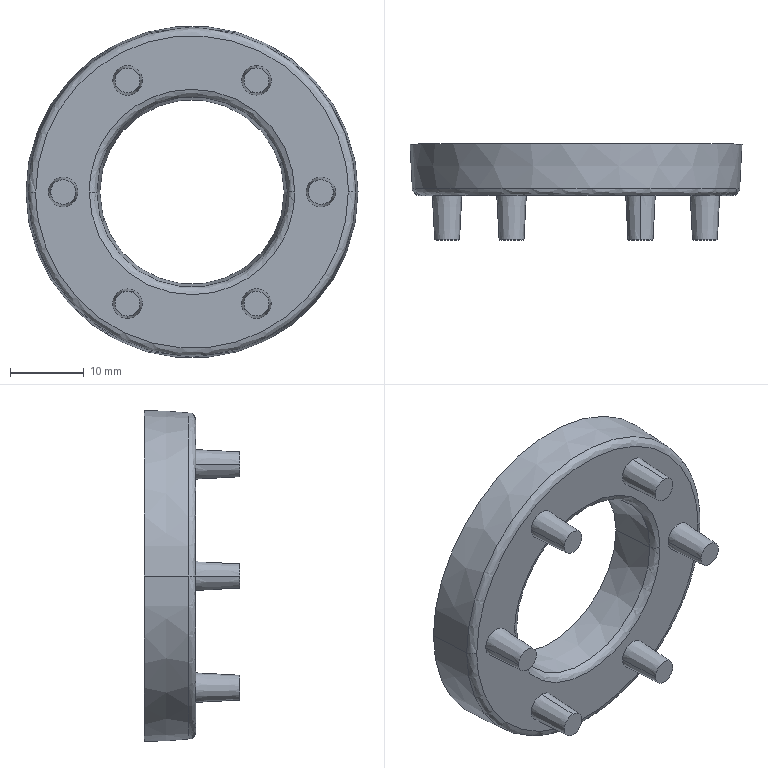Part | SolidWorks | features BaseBody 1 | 1 solid | 28 faces | box 45 x 13 x 45 mm | volume 7724 mm3 | cone 16 | plane 8 | spline 4
STEP:
#1=CARTESIAN_POINT('',(-13.922,-55.,0.));
#2=VERTEX_POINT('',#1);
#3=CARTESIAN_POINT('',(13.922,-55.,0.));
#4=VERTEX_POINT('',#3);
#5=CARTESIAN_POINT('',(-13.922,-55.,0.));
#6=CARTESIAN_POINT('',(-13.922,-55.,-27.844));
#7=CARTESIAN_POINT('',(13.922,-55.,-27.844));
#8=CARTESIAN_POINT('',(13.922,-55.,0.));
#9=(BOUNDED_CURVE()B_SPLINE_CURVE(3,(#5,#6,#7,#8),.UNSPECIFIED.,.F.,.T.)B_SPLINE_CURVE_WITH_KNOTS((4,4),(0.,0.5),.UNSPECIFIED.)CURVE()GEOMETRIC_REPRESENTATION_ITEM()RATIONAL_B_SPLINE_CURVE((1.,0.3333,0.3333,1.))REPRESENTATION_ITEM(''));
#10=EDGE_CURVE('',#2,#4,#9,.T.);
#11=ORIENTED_EDGE('',*,*,#10,.T.);
#12=CARTESIAN_POINT('',(12.924,-54.07,0.));
#13=VERTEX_POINT('',#12);
#14=CARTESIAN_POINT('',(13.922,-54.,0.));
#15=DIRECTION('',(0.,0.,-1.));
#16=DIRECTION('',(1.,0.,0.));
#17=AXIS2_PLACEMENT_3D('',#14,#15,#16);
#18=CIRCLE('',#17,1.);
#19=EDGE_CURVE('',#4,#13,#18,.T.);
#20=ORIENTED_EDGE('',*,*,#19,.T.);
#21=CARTESIAN_POINT('',(-12.924,-54.07,0.));
#22=VERTEX_POINT('',#21);
#23=CARTESIAN_POINT('',(0.,-54.07,0.));
#24=DIRECTION('',(0.,1.,0.));
#25=DIRECTION('',(1.,0.,0.));
#26=AXIS2_PLACEMENT_3D('',#23,#24,#25);
#27=CIRCLE('',#26,12.924);
#28=EDGE_CURVE('',#13,#22,#27,.T.);
#29=ORIENTED_EDGE('',*,*,#28,.T.);
#30=CARTESIAN_POINT('',(-13.922,-54.,0.));
#31=DIRECTION('',(0.,0.,1.));
#32=DIRECTION('',(-1.,0.,0.));
#33=AXIS2_PLACEMENT_3D('',#30,#31,#32);
#34=CIRCLE('',#33,1.);
#35=EDGE_CURVE('',#2,#22,#34,.T.);
#36=ORIENTED_EDGE('',*,*,#35,.F.);
#37=EDGE_LOOP('',(#11,#20,#29,#36));
#38=FACE_OUTER_BOUND('',#37,.T.);
#39=CARTESIAN_POINT('',(13.922,-55.,0.));
#40=CARTESIAN_POINT('',(13.922,-55.,-27.844));
#41=CARTESIAN_POINT('',(-13.922,-55.,-27.844));
#42=CARTESIAN_POINT('',(-13.922,-55.,0.));
#43=CARTESIAN_POINT('',(13.368,-55.,0.));
#44=CARTESIAN_POINT('',(13.368,-55.,-26.736));
#45=CARTESIAN_POINT('',(-13.368,-55.,-26.736));
#46=CARTESIAN_POINT('',(-13.368,-55.,0.));
#47=CARTESIAN_POINT('',(12.963,-54.622,0.));
#48=CARTESIAN_POINT('',(12.963,-54.622,-25.926));
#49=CARTESIAN_POINT('',(-12.963,-54.622,-25.926));
#50=CARTESIAN_POINT('',(-12.963,-54.622,0.));
#51=CARTESIAN_POINT('',(12.924,-54.07,0.));
#52=CARTESIAN_POINT('',(12.924,-54.07,-25.849));
#53=CARTESIAN_POINT('',(-12.924,-54.07,-25.849));
#54=CARTESIAN_POINT('',(-12.924,-54.07,0.));
#55=(BOUNDED_SURFACE()B_SPLINE_SURFACE(3,3,((#39,#40,#41,#42),(#43,#44,#45,#46),(#47,#48,#49,#50),(#51,#52,#53,#54)),.UNSPECIFIED.,.F.,.F.,.F.)B_SPLINE_SURFACE_WITH_KNOTS((4,4),(4,4),(0.,1.),(0.,1.),.UNSPECIFIED.)GEOMETRIC_REPRESENTATION_ITEM()RATIONAL_B_SPLINE_SURFACE(((1.,0.3333,0.3333,1.),(0.8209,0.2736,0.2736,0.8209),(0.8209,0.2736,0.2736,0.8209),(1.,0.3333,0.3333,1.)))REPRESENTATION_ITEM('')SURFACE());
#56=ADVANCED_FACE('',(#38),#55,.T.);
#57=CARTESIAN_POINT('',(22.183,-54.052,0.));
#58=VERTEX_POINT('',#57);
#59=CARTESIAN_POINT('',(-22.183,-54.052,0.));
#60=VERTEX_POINT('',#59);
#61=CARTESIAN_POINT('',(0.,-54.052,0.));
#62=DIRECTION('',(0.,1.,0.));
#63=DIRECTION('',(-1.,0.,0.));
#64=AXIS2_PLACEMENT_3D('',#61,#62,#63);
#65=CIRCLE('',#64,22.183);
#66=EDGE_CURVE('',#58,#60,#65,.T.);
#67=ORIENTED_EDGE('',*,*,#66,.F.);
#68=CARTESIAN_POINT('',(21.184,-55.,0.));
#69=VERTEX_POINT('',#68);
#70=CARTESIAN_POINT('',(21.184,-54.,0.));
#71=DIRECTION('',(0.,0.,-1.));
#72=DIRECTION('',(1.,0.,0.));
#73=AXIS2_PLACEMENT_3D('',#70,#71,#72);
#74=CIRCLE('',#73,1.);
#75=EDGE_CURVE('',#58,#69,#74,.T.);
#76=ORIENTED_EDGE('',*,*,#75,.T.);
#77=CARTESIAN_POINT('',(-21.184,-55.,0.));
#78=VERTEX_POINT('',#77);
#79=CARTESIAN_POINT('',(21.184,-55.,0.));
#80=CARTESIAN_POINT('',(21.184,-55.,-42.368));
#81=CARTESIAN_POINT('',(-21.184,-55.,-42.368));
#82=CARTESIAN_POINT('',(-21.184,-55.,0.));
#83=(BOUNDED_CURVE()B_SPLINE_CURVE(3,(#79,#80,#81,#82),.UNSPECIFIED.,.F.,.F.)B_SPLINE_CURVE_WITH_KNOTS((4,4),(0.5,1.),.UNSPECIFIED.)CURVE()GEOMETRIC_REPRESENTATION_ITEM()RATIONAL_B_SPLINE_CURVE((1.,0.3333,0.3333,1.))REPRESENTATION_ITEM(''));
#84=EDGE_CURVE('',#69,#78,#83,.T.);
#85=ORIENTED_EDGE('',*,*,#84,.T.);
#86=CARTESIAN_POINT('',(-21.184,-54.,0.));
#87=DIRECTION('',(0.,0.,1.));
#88=DIRECTION('',(-1.,0.,0.));
#89=AXIS2_PLACEMENT_3D('',#86,#87,#88);
#90=CIRCLE('',#89,1.);
#91=EDGE_CURVE('',#60,#78,#90,.T.);
#92=ORIENTED_EDGE('',*,*,#91,.F.);
#93=EDGE_LOOP('',(#67,#76,#85,#92));
#94=FACE_OUTER_BOUND('',#93,.T.);
#95=CARTESIAN_POINT('',(22.183,-54.052,0.));
#96=CARTESIAN_POINT('',(22.183,-54.052,-44.366));
#97=CARTESIAN_POINT('',(-22.183,-54.052,-44.366));
#98=CARTESIAN_POINT('',(-22.183,-54.052,0.));
#99=CARTESIAN_POINT('',(22.153,-54.613,0.));
#100=CARTESIAN_POINT('',(22.153,-54.613,-44.307));
#101=CARTESIAN_POINT('',(-22.153,-54.613,-44.307));
#102=CARTESIAN_POINT('',(-22.153,-54.613,0.));
#103=CARTESIAN_POINT('',(21.746,-55.,0.));
#104=CARTESIAN_POINT('',(21.746,-55.,-43.492));
#105=CARTESIAN_POINT('',(-21.746,-55.,-43.492));
#106=CARTESIAN_POINT('',(-21.746,-55.,0.));
#107=CARTESIAN_POINT('',(21.184,-55.,0.));
#108=CARTESIAN_POINT('',(21.184,-55.,-42.368));
#109=CARTESIAN_POINT('',(-21.184,-55.,-42.368));
#110=CARTESIAN_POINT('',(-21.184,-55.,0.));
#111=(BOUNDED_SURFACE()B_SPLINE_SURFACE(3,3,((#95,#96,#97,#98),(#99,#100,#101,#102),(#103,#104,#105,#106),(#107,#108,#109,#110)),.UNSPECIFIED.,.F.,.F.,.F.)B_SPLINE_SURFACE_WITH_KNOTS((4,4),(4,4),(0.,1.),(0.,1.),.UNSPECIFIED.)GEOMETRIC_REPRESENTATION_ITEM()RATIONAL_B_SPLINE_SURFACE(((1.,0.3333,0.3333,1.),(0.8169,0.2723,0.2723,0.8169),(0.8169,0.2723,0.2723,0.8169),(1.,0.3333,0.3333,1.)))REPRESENTATION_ITEM('')SURFACE());
#112=ADVANCED_FACE('',(#94),#111,.T.);
#113=CARTESIAN_POINT('',(-12.5,-48.,0.));
#114=VERTEX_POINT('',#113);
#115=CARTESIAN_POINT('',(12.5,-48.,0.));
#116=VERTEX_POINT('',#115);
#117=CARTESIAN_POINT('',(0.,-48.,0.));
#118=DIRECTION('',(0.,-1.,0.));
#119=DIRECTION('',(1.,0.,0.));
#120=AXIS2_PLACEMENT_3D('',#117,#118,#119);
#121=CIRCLE('',#120,12.5);
#122=EDGE_CURVE('',#114,#116,#121,.T.);
#123=ORIENTED_EDGE('',*,*,#122,.F.);
#124=CARTESIAN_POINT('',(-12.924,-54.07,0.));
#125=DIRECTION('',(-0.06976,-0.9976,0.));
#126=VECTOR('',#125,1000.);
#127=LINE('',#124,#126);
#128=EDGE_CURVE('',#114,#22,#127,.T.);
#129=ORIENTED_EDGE('',*,*,#128,.T.);
#130=ORIENTED_EDGE('',*,*,#28,.F.);
#131=CARTESIAN_POINT('',(12.924,-54.07,0.));
#132=DIRECTION('',(0.06976,-0.9976,0.));
#133=VECTOR('',#132,1000.);
#134=LINE('',#131,#133);
#135=EDGE_CURVE('',#116,#13,#134,.T.);
#136=ORIENTED_EDGE('',*,*,#135,.F.);
#137=EDGE_LOOP('',(#123,#129,#130,#136));
#138=FACE_OUTER_BOUND('',#137,.T.);
#139=CARTESIAN_POINT('',(0.,-54.07,0.));
#140=DIRECTION('',(0.,-1.,0.));
#141=DIRECTION('',(1.,0.,0.));
#142=AXIS2_PLACEMENT_3D('',#139,#140,#141);
#143=CONICAL_SURFACE('',#142,12.924,0.06981);
#144=ADVANCED_FACE('',(#138),#143,.F.);
#145=CARTESIAN_POINT('',(0.,-54.052,0.));
#146=DIRECTION('',(0.,1.,0.));
#147=DIRECTION('',(-1.,0.,0.));
#148=AXIS2_PLACEMENT_3D('',#145,#146,#147);
#149=CIRCLE('',#148,22.183);
#150=EDGE_CURVE('',#60,#58,#149,.T.);
#151=ORIENTED_EDGE('',*,*,#150,.T.);
#152=CARTESIAN_POINT('',(22.5,-48.,0.));
#153=VERTEX_POINT('',#152);
#154=CARTESIAN_POINT('',(22.5,-48.,0.));
#155=DIRECTION('',(0.05234,0.9986,0.));
#156=VECTOR('',#155,1000.);
#157=LINE('',#154,#156);
#158=EDGE_CURVE('',#58,#153,#157,.T.);
#159=ORIENTED_EDGE('',*,*,#158,.T.);
#160=CARTESIAN_POINT('',(-22.5,-48.,0.));
#161=VERTEX_POINT('',#160);
#162=CARTESIAN_POINT('',(0.,-48.,0.));
#163=DIRECTION('',(0.,1.,0.));
#164=DIRECTION('',(-1.,0.,0.));
#165=AXIS2_PLACEMENT_3D('',#162,#163,#164);
#166=CIRCLE('',#165,22.5);
#167=EDGE_CURVE('',#161,#153,#166,.T.);
#168=ORIENTED_EDGE('',*,*,#167,.F.);
#169=CARTESIAN_POINT('',(-22.5,-48.,0.));
#170=DIRECTION('',(-0.05234,0.9986,0.));
#171=VECTOR('',#170,1000.);
#172=LINE('',#169,#171);
#173=EDGE_CURVE('',#60,#161,#172,.T.);
#174=ORIENTED_EDGE('',*,*,#173,.F.);
#175=EDGE_LOOP('',(#151,#159,#168,#174));
#176=FACE_OUTER_BOUND('',#175,.T.);
#177=CARTESIAN_POINT('',(0.,-48.,0.));
#178=DIRECTION('',(0.,1.,0.));
#179=DIRECTION('',(-1.,0.,0.));
#180=AXIS2_PLACEMENT_3D('',#177,#178,#179);
#181=CONICAL_SURFACE('',#180,22.5,0.05236);
#182=ADVANCED_FACE('',(#176),#181,.T.);
#183=CARTESIAN_POINT('',(-10.422,-61.,15.133));
#184=VERTEX_POINT('',#183);
#185=CARTESIAN_POINT('',(-7.051,-61.,15.133));
#186=VERTEX_POINT('',#185);
#187=CARTESIAN_POINT('',(-8.737,-61.,15.133));
#188=DIRECTION('',(0.,1.,0.));
#189=DIRECTION('',(-1.,0.,0.));
#190=AXIS2_PLACEMENT_3D('',#187,#188,#189);
#191=CIRCLE('',#190,1.686);
#192=EDGE_CURVE('',#184,#186,#191,.T.);
#193=ORIENTED_EDGE('',*,*,#192,.T.);
#194=CARTESIAN_POINT('',(-6.737,-55.,15.133));
#195=VERTEX_POINT('',#194);
#196=CARTESIAN_POINT('',(-6.737,-55.,15.133));
#197=DIRECTION('',(0.05234,0.9986,0.));
#198=VECTOR('',#197,1000.);
#199=LINE('',#196,#198);
#200=EDGE_CURVE('',#186,#195,#199,.T.);
#201=ORIENTED_EDGE('',*,*,#200,.T.);
#202=CARTESIAN_POINT('',(-10.737,-55.,15.133));
#203=VERTEX_POINT('',#202);
#204=CARTESIAN_POINT('',(-8.737,-55.,15.133));
#205=DIRECTION('',(0.,1.,0.));
#206=DIRECTION('',(-1.,0.,0.));
#207=AXIS2_PLACEMENT_3D('',#204,#205,#206);
#208=CIRCLE('',#207,2.);
#209=EDGE_CURVE('',#203,#195,#208,.T.);
#210=ORIENTED_EDGE('',*,*,#209,.F.);
#211=CARTESIAN_POINT('',(-10.737,-55.,15.133));
#212=DIRECTION('',(-0.05234,0.9986,0.));
#213=VECTOR('',#212,1000.);
#214=LINE('',#211,#213);
#215=EDGE_CURVE('',#184,#203,#214,.T.);
#216=ORIENTED_EDGE('',*,*,#215,.F.);
#217=EDGE_LOOP('',(#193,#201,#210,#216));
#218=FACE_OUTER_BOUND('',#217,.T.);
#219=CARTESIAN_POINT('',(-8.737,-55.,15.133));
#220=DIRECTION('',(0.,1.,0.));
#221=DIRECTION('',(-1.,0.,0.));
#222=AXIS2_PLACEMENT_3D('',#219,#220,#221);
#223=CONICAL_SURFACE('',#222,2.,0.05236);
#224=ADVANCED_FACE('',(#218),#223,.T.);
#225=CARTESIAN_POINT('',(7.051,-61.,-15.133));
#226=VERTEX_POINT('',#225);
#227=CARTESIAN_POINT('',(10.422,-61.,-15.133));
#228=VERTEX_POINT('',#227);
#229=CARTESIAN_POINT('',(8.737,-61.,-15.133));
#230=DIRECTION('',(0.,1.,0.));
#231=DIRECTION('',(-1.,0.,0.));
#232=AXIS2_PLACEMENT_3D('',#229,#230,#231);
#233=CIRCLE('',#232,1.686);
#234=EDGE_CURVE('',#226,#228,#233,.T.);
#235=ORIENTED_EDGE('',*,*,#234,.T.);
#236=CARTESIAN_POINT('',(10.737,-55.,-15.133));
#237=VERTEX_POINT('',#236);
#238=CARTESIAN_POINT('',(10.737,-55.,-15.133));
#239=DIRECTION('',(0.05234,0.9986,0.));
#240=VECTOR('',#239,1000.);
#241=LINE('',#238,#240);
#242=EDGE_CURVE('',#228,#237,#241,.T.);
#243=ORIENTED_EDGE('',*,*,#242,.T.);
#244=CARTESIAN_POINT('',(6.737,-55.,-15.133));
#245=VERTEX_POINT('',#244);
#246=CARTESIAN_POINT('',(8.737,-55.,-15.133));
#247=DIRECTION('',(0.,1.,0.));
#248=DIRECTION('',(-1.,0.,0.));
#249=AXIS2_PLACEMENT_3D('',#246,#247,#248);
#250=CIRCLE('',#249,2.);
#251=EDGE_CURVE('',#245,#237,#250,.T.);
#252=ORIENTED_EDGE('',*,*,#251,.F.);
#253=CARTESIAN_POINT('',(6.737,-55.,-15.133));
#254=DIRECTION('',(-0.05234,0.9986,0.));
#255=VECTOR('',#254,1000.);
#256=LINE('',#253,#255);
#257=EDGE_CURVE('',#226,#245,#256,.T.);
#258=ORIENTED_EDGE('',*,*,#257,.F.);
#259=EDGE_LOOP('',(#235,#243,#252,#258));
#260=FACE_OUTER_BOUND('',#259,.T.);
#261=CARTESIAN_POINT('',(8.737,-55.,-15.133));
#262=DIRECTION('',(0.,1.,0.));
#263=DIRECTION('',(-1.,0.,0.));
#264=AXIS2_PLACEMENT_3D('',#261,#262,#263);
#265=CONICAL_SURFACE('',#264,2.,0.05236);
#266=ADVANCED_FACE('',(#260),#265,.T.);
#267=CARTESIAN_POINT('',(8.737,-61.,16.818));
#268=VERTEX_POINT('',#267);
#269=CARTESIAN_POINT('',(8.737,-61.,13.447));
#270=VERTEX_POINT('',#269);
#271=CARTESIAN_POINT('',(8.737,-61.,15.133));
#272=DIRECTION('',(0.,1.,0.));
#273=DIRECTION('',(0.,0.,1.));
#274=AXIS2_PLACEMENT_3D('',#271,#272,#273);
#275=CIRCLE('',#274,1.686);
#276=EDGE_CURVE('',#268,#270,#275,.T.);
#277=ORIENTED_EDGE('',*,*,#276,.T.);
#278=CARTESIAN_POINT('',(8.737,-55.,13.133));
#279=VERTEX_POINT('',#278);
#280=CARTESIAN_POINT('',(8.737,-55.,13.133));
#281=DIRECTION('',(0.,0.9986,-0.05234));
#282=VECTOR('',#281,1000.);
#283=LINE('',#280,#282);
#284=EDGE_CURVE('',#270,#279,#283,.T.);
#285=ORIENTED_EDGE('',*,*,#284,.T.);
#286=CARTESIAN_POINT('',(8.737,-55.,17.133));
#287=VERTEX_POINT('',#286);
#288=CARTESIAN_POINT('',(8.737,-55.,15.133));
#289=DIRECTION('',(0.,1.,0.));
#290=DIRECTION('',(0.,0.,1.));
#291=AXIS2_PLACEMENT_3D('',#288,#289,#290);
#292=CIRCLE('',#291,2.);
#293=EDGE_CURVE('',#287,#279,#292,.T.);
#294=ORIENTED_EDGE('',*,*,#293,.F.);
#295=CARTESIAN_POINT('',(8.737,-55.,17.133));
#296=DIRECTION('',(0.,0.9986,0.05234));
#297=VECTOR('',#296,1000.);
#298=LINE('',#295,#297);
#299=EDGE_CURVE('',#268,#287,#298,.T.);
#300=ORIENTED_EDGE('',*,*,#299,.F.);
#301=EDGE_LOOP('',(#277,#285,#294,#300));
#302=FACE_OUTER_BOUND('',#301,.T.);
#303=CARTESIAN_POINT('',(8.737,-55.,15.133));
#304=DIRECTION('',(0.,1.,0.));
#305=DIRECTION('',(0.,0.,1.));
#306=AXIS2_PLACEMENT_3D('',#303,#304,#305);
#307=CONICAL_SURFACE('',#306,2.,0.05236);
#308=ADVANCED_FACE('',(#302),#307,.T.);
#309=CARTESIAN_POINT('',(15.788,-61.,0.));
#310=VERTEX_POINT('',#309);
#311=CARTESIAN_POINT('',(19.159,-61.,0.));
#312=VERTEX_POINT('',#311);
#313=CARTESIAN_POINT('',(17.474,-61.,0.));
#314=DIRECTION('',(0.,1.,0.));
#315=DIRECTION('',(-1.,0.,0.));
#316=AXIS2_PLACEMENT_3D('',#313,#314,#315);
#317=CIRCLE('',#316,1.686);
#318=EDGE_CURVE('',#310,#312,#317,.T.);
#319=ORIENTED_EDGE('',*,*,#318,.T.);
#320=CARTESIAN_POINT('',(19.474,-55.,0.));
#321=VERTEX_POINT('',#320);
#322=CARTESIAN_POINT('',(19.474,-55.,0.));
#323=DIRECTION('',(0.05234,0.9986,0.));
#324=VECTOR('',#323,1000.);
#325=LINE('',#322,#324);
#326=EDGE_CURVE('',#312,#321,#325,.T.);
#327=ORIENTED_EDGE('',*,*,#326,.T.);
#328=CARTESIAN_POINT('',(15.474,-55.,0.));
#329=VERTEX_POINT('',#328);
#330=CARTESIAN_POINT('',(17.474,-55.,0.));
#331=DIRECTION('',(0.,1.,0.));
#332=DIRECTION('',(-1.,0.,0.));
#333=AXIS2_PLACEMENT_3D('',#330,#331,#332);
#334=CIRCLE('',#333,2.);
#335=EDGE_CURVE('',#329,#321,#334,.T.);
#336=ORIENTED_EDGE('',*,*,#335,.F.);
#337=CARTESIAN_POINT('',(15.474,-55.,0.));
#338=DIRECTION('',(-0.05234,0.9986,0.));
#339=VECTOR('',#338,1000.);
#340=LINE('',#337,#339);
#341=EDGE_CURVE('',#310,#329,#340,.T.);
#342=ORIENTED_EDGE('',*,*,#341,.F.);
#343=EDGE_LOOP('',(#319,#327,#336,#342));
#344=FACE_OUTER_BOUND('',#343,.T.);
#345=CARTESIAN_POINT('',(17.474,-55.,0.));
#346=DIRECTION('',(0.,1.,0.));
#347=DIRECTION('',(-1.,0.,0.));
#348=AXIS2_PLACEMENT_3D('',#345,#346,#347);
#349=CONICAL_SURFACE('',#348,2.,0.05236);
#350=ADVANCED_FACE('',(#344),#349,.T.);
#351=CARTESIAN_POINT('',(-19.159,-61.,0.));
#352=VERTEX_POINT('',#351);
#353=CARTESIAN_POINT('',(-15.788,-61.,0.));
#354=VERTEX_POINT('',#353);
#355=CARTESIAN_POINT('',(-17.474,-61.,0.));
#356=DIRECTION('',(0.,1.,0.));
#357=DIRECTION('',(-1.,0.,0.));
#358=AXIS2_PLACEMENT_3D('',#355,#356,#357);
#359=CIRCLE('',#358,1.686);
#360=EDGE_CURVE('',#352,#354,#359,.T.);
#361=ORIENTED_EDGE('',*,*,#360,.T.);
#362=CARTESIAN_POINT('',(-15.474,-55.,0.));
#363=VERTEX_POINT('',#362);
#364=CARTESIAN_POINT('',(-15.474,-55.,0.));
#365=DIRECTION('',(0.05234,0.9986,0.));
#366=VECTOR('',#365,1000.);
#367=LINE('',#364,#366);
#368=EDGE_CURVE('',#354,#363,#367,.T.);
#369=ORIENTED_EDGE('',*,*,#368,.T.);
#370=CARTESIAN_POINT('',(-19.474,-55.,0.));
#371=VERTEX_POINT('',#370);
#372=CARTESIAN_POINT('',(-17.474,-55.,0.));
#373=DIRECTION('',(0.,1.,0.));
#374=DIRECTION('',(-1.,0.,0.));
#375=AXIS2_PLACEMENT_3D('',#372,#373,#374);
#376=CIRCLE('',#375,2.);
#377=EDGE_CURVE('',#371,#363,#376,.T.);
#378=ORIENTED_EDGE('',*,*,#377,.F.);
#379=CARTESIAN_POINT('',(-19.474,-55.,0.));
#380=DIRECTION('',(-0.05234,0.9986,0.));
#381=VECTOR('',#380,1000.);
#382=LINE('',#379,#381);
#383=EDGE_CURVE('',#352,#371,#382,.T.);
#384=ORIENTED_EDGE('',*,*,#383,.F.);
#385=EDGE_LOOP('',(#361,#369,#378,#384));
#386=FACE_OUTER_BOUND('',#385,.T.);
#387=CARTESIAN_POINT('',(-17.474,-55.,0.));
#388=DIRECTION('',(0.,1.,0.));
#389=DIRECTION('',(-1.,0.,0.));
#390=AXIS2_PLACEMENT_3D('',#387,#388,#389);
#391=CONICAL_SURFACE('',#390,2.,0.05236);
#392=ADVANCED_FACE('',(#386),#391,.T.);
#393=CARTESIAN_POINT('',(-8.737,-61.,-13.447));
#394=VERTEX_POINT('',#393);
#395=CARTESIAN_POINT('',(-8.737,-61.,-16.818));
#396=VERTEX_POINT('',#395);
#397=CARTESIAN_POINT('',(-8.737,-61.,-15.133));
#398=DIRECTION('',(0.,1.,0.));
#399=DIRECTION('',(0.,0.,1.));
#400=AXIS2_PLACEMENT_3D('',#397,#398,#399);
#401=CIRCLE('',#400,1.686);
#402=EDGE_CURVE('',#394,#396,#401,.T.);
#403=ORIENTED_EDGE('',*,*,#402,.T.);
#404=CARTESIAN_POINT('',(-8.737,-55.,-17.133));
#405=VERTEX_POINT('',#404);
#406=CARTESIAN_POINT('',(-8.737,-55.,-17.133));
#407=DIRECTION('',(0.,0.9986,-0.05234));
#408=VECTOR('',#407,1000.);
#409=LINE('',#406,#408);
#410=EDGE_CURVE('',#396,#405,#409,.T.);
#411=ORIENTED_EDGE('',*,*,#410,.T.);
#412=CARTESIAN_POINT('',(-8.737,-55.,-13.133));
#413=VERTEX_POINT('',#412);
#414=CARTESIAN_POINT('',(-8.737,-55.,-15.133));
#415=DIRECTION('',(0.,1.,0.));
#416=DIRECTION('',(0.,0.,1.));
#417=AXIS2_PLACEMENT_3D('',#414,#415,#416);
#418=CIRCLE('',#417,2.);
#419=EDGE_CURVE('',#413,#405,#418,.T.);
#420=ORIENTED_EDGE('',*,*,#419,.F.);
#421=CARTESIAN_POINT('',(-8.737,-55.,-13.133));
#422=DIRECTION('',(0.,0.9986,0.05234));
#423=VECTOR('',#422,1000.);
#424=LINE('',#421,#423);
#425=EDGE_CURVE('',#394,#413,#424,.T.);
#426=ORIENTED_EDGE('',*,*,#425,.F.);
#427=EDGE_LOOP('',(#403,#411,#420,#426));
#428=FACE_OUTER_BOUND('',#427,.T.);
#429=CARTESIAN_POINT('',(-8.737,-55.,-15.133));
#430=DIRECTION('',(0.,1.,0.));
#431=DIRECTION('',(0.,0.,1.));
#432=AXIS2_PLACEMENT_3D('',#429,#430,#431);
#433=CONICAL_SURFACE('',#432,2.,0.05236);
#434=ADVANCED_FACE('',(#428),#433,.T.);
#435=CARTESIAN_POINT('',(0.,-48.,0.));
#436=DIRECTION('',(0.,-1.,0.));
#437=DIRECTION('',(1.,0.,0.));
#438=AXIS2_PLACEMENT_3D('',#435,#436,#437);
#439=CIRCLE('',#438,12.5);
#440=EDGE_CURVE('',#116,#114,#439,.T.);
#441=ORIENTED_EDGE('',*,*,#440,.T.);
#442=ORIENTED_EDGE('',*,*,#122,.T.);
#443=EDGE_LOOP('',(#441,#442));
#444=FACE_BOUND('',#443,.T.);
#445=ORIENTED_EDGE('',*,*,#167,.T.);
#446=CARTESIAN_POINT('',(0.,-48.,0.));
#447=DIRECTION('',(0.,1.,0.));
#448=DIRECTION('',(-1.,0.,0.));
#449=AXIS2_PLACEMENT_3D('',#446,#447,#448);
#450=CIRCLE('',#449,22.5);
#451=EDGE_CURVE('',#153,#161,#450,.T.);
#452=ORIENTED_EDGE('',*,*,#451,.T.);
#453=EDGE_LOOP('',(#445,#452));
#454=FACE_OUTER_BOUND('',#453,.T.);
#455=CARTESIAN_POINT('',(0.,-48.,-12.5));
#456=DIRECTION('',(0.,1.,0.));
#457=DIRECTION('',(0.,0.,1.));
#458=AXIS2_PLACEMENT_3D('',#455,#456,#457);
#459=PLANE('',#458);
#460=ADVANCED_FACE('',(#444,#454),#459,.T.);
#461=ORIENTED_EDGE('',*,*,#128,.F.);
#462=ORIENTED_EDGE('',*,*,#440,.F.);
#463=ORIENTED_EDGE('',*,*,#135,.T.);
#464=CARTESIAN_POINT('',(0.,-54.07,0.));
#465=DIRECTION('',(0.,1.,0.));
#466=DIRECTION('',(1.,0.,0.));
#467=AXIS2_PLACEMENT_3D('',#464,#465,#466);
#468=CIRCLE('',#467,12.924);
#469=EDGE_CURVE('',#22,#13,#468,.T.);
#470=ORIENTED_EDGE('',*,*,#469,.F.);
#471=EDGE_LOOP('',(#461,#462,#463,#470));
#472=FACE_OUTER_BOUND('',#471,.T.);
#473=CARTESIAN_POINT('',(0.,-54.07,0.));
#474=DIRECTION('',(0.,-1.,0.));
#475=DIRECTION('',(1.,0.,0.));
#476=AXIS2_PLACEMENT_3D('',#473,#474,#475);
#477=CONICAL_SURFACE('',#476,12.924,0.06981);
#478=ADVANCED_FACE('',(#472),#477,.F.);
#479=ORIENTED_EDGE('',*,*,#158,.F.);
#480=ORIENTED_EDGE('',*,*,#66,.T.);
#481=ORIENTED_EDGE('',*,*,#173,.T.);
#482=ORIENTED_EDGE('',*,*,#451,.F.);
#483=EDGE_LOOP('',(#479,#480,#481,#482));
#484=FACE_OUTER_BOUND('',#483,.T.);
#485=CARTESIAN_POINT('',(0.,-48.,0.));
#486=DIRECTION('',(0.,1.,0.));
#487=DIRECTION('',(-1.,0.,0.));
#488=AXIS2_PLACEMENT_3D('',#485,#486,#487);
#489=CONICAL_SURFACE('',#488,22.5,0.05236);
#490=ADVANCED_FACE('',(#484),#489,.T.);
#491=ORIENTED_EDGE('',*,*,#19,.F.);
#492=CARTESIAN_POINT('',(13.922,-55.,0.));
#493=CARTESIAN_POINT('',(13.922,-55.,27.844));
#494=CARTESIAN_POINT('',(-13.922,-55.,27.844));
#495=CARTESIAN_POINT('',(-13.922,-55.,0.));
#496=(BOUNDED_CURVE()B_SPLINE_CURVE(3,(#492,#493,#494,#495),.UNSPECIFIED.,.F.,.F.)B_SPLINE_CURVE_WITH_KNOTS((4,4),(0.5,1.),.UNSPECIFIED.)CURVE()GEOMETRIC_REPRESENTATION_ITEM()RATIONAL_B_SPLINE_CURVE((1.,0.3333,0.3333,1.))REPRESENTATION_ITEM(''));
#497=EDGE_CURVE('',#4,#2,#496,.T.);
#498=ORIENTED_EDGE('',*,*,#497,.T.);
#499=ORIENTED_EDGE('',*,*,#35,.T.);
#500=ORIENTED_EDGE('',*,*,#469,.T.);
#501=EDGE_LOOP('',(#491,#498,#499,#500));
#502=FACE_OUTER_BOUND('',#501,.T.);
#503=CARTESIAN_POINT('',(-13.922,-55.,0.));
#504=CARTESIAN_POINT('',(-13.922,-55.,27.844));
#505=CARTESIAN_POINT('',(13.922,-55.,27.844));
#506=CARTESIAN_POINT('',(13.922,-55.,0.));
#507=CARTESIAN_POINT('',(-13.368,-55.,0.));
#508=CARTESIAN_POINT('',(-13.368,-55.,26.736));
#509=CARTESIAN_POINT('',(13.368,-55.,26.736));
#510=CARTESIAN_POINT('',(13.368,-55.,0.));
#511=CARTESIAN_POINT('',(-12.963,-54.622,0.));
#512=CARTESIAN_POINT('',(-12.963,-54.622,25.926));
#513=CARTESIAN_POINT('',(12.963,-54.622,25.926));
#514=CARTESIAN_POINT('',(12.963,-54.622,0.));
#515=CARTESIAN_POINT('',(-12.924,-54.07,0.));
#516=CARTESIAN_POINT('',(-12.924,-54.07,25.849));
#517=CARTESIAN_POINT('',(12.924,-54.07,25.849));
#518=CARTESIAN_POINT('',(12.924,-54.07,0.));
#519=(BOUNDED_SURFACE()B_SPLINE_SURFACE(3,3,((#503,#504,#505,#506),(#507,#508,#509,#510),(#511,#512,#513,#514),(#515,#516,#517,#518)),.UNSPECIFIED.,.F.,.F.,.F.)B_SPLINE_SURFACE_WITH_KNOTS((4,4),(4,4),(0.,1.),(0.,1.),.UNSPECIFIED.)GEOMETRIC_REPRESENTATION_ITEM()RATIONAL_B_SPLINE_SURFACE(((1.,0.3333,0.3333,1.),(0.8209,0.2736,0.2736,0.8209),(0.8209,0.2736,0.2736,0.8209),(1.,0.3333,0.3333,1.)))REPRESENTATION_ITEM('')SURFACE());
#520=ADVANCED_FACE('',(#502),#519,.T.);
#521=ORIENTED_EDGE('',*,*,#75,.F.);
#522=ORIENTED_EDGE('',*,*,#150,.F.);
#523=ORIENTED_EDGE('',*,*,#91,.T.);
#524=CARTESIAN_POINT('',(-21.184,-55.,0.));
#525=CARTESIAN_POINT('',(-21.184,-55.,42.368));
#526=CARTESIAN_POINT('',(21.184,-55.,42.368));
#527=CARTESIAN_POINT('',(21.184,-55.,0.));
#528=(BOUNDED_CURVE()B_SPLINE_CURVE(3,(#524,#525,#526,#527),.UNSPECIFIED.,.F.,.F.)B_SPLINE_CURVE_WITH_KNOTS((4,4),(0.,0.5),.UNSPECIFIED.)CURVE()GEOMETRIC_REPRESENTATION_ITEM()RATIONAL_B_SPLINE_CURVE((1.,0.3333,0.3333,1.))REPRESENTATION_ITEM(''));
#529=EDGE_CURVE('',#78,#69,#528,.T.);
#530=ORIENTED_EDGE('',*,*,#529,.T.);
#531=EDGE_LOOP('',(#521,#522,#523,#530));
#532=FACE_OUTER_BOUND('',#531,.T.);
#533=CARTESIAN_POINT('',(-22.183,-54.052,0.));
#534=CARTESIAN_POINT('',(-22.183,-54.052,44.366));
#535=CARTESIAN_POINT('',(22.183,-54.052,44.366));
#536=CARTESIAN_POINT('',(22.183,-54.052,0.));
#537=CARTESIAN_POINT('',(-22.153,-54.613,0.));
#538=CARTESIAN_POINT('',(-22.153,-54.613,44.307));
#539=CARTESIAN_POINT('',(22.153,-54.613,44.307));
#540=CARTESIAN_POINT('',(22.153,-54.613,0.));
#541=CARTESIAN_POINT('',(-21.746,-55.,0.));
#542=CARTESIAN_POINT('',(-21.746,-55.,43.492));
#543=CARTESIAN_POINT('',(21.746,-55.,43.492));
#544=CARTESIAN_POINT('',(21.746,-55.,0.));
#545=CARTESIAN_POINT('',(-21.184,-55.,0.));
#546=CARTESIAN_POINT('',(-21.184,-55.,42.368));
#547=CARTESIAN_POINT('',(21.184,-55.,42.368));
#548=CARTESIAN_POINT('',(21.184,-55.,0.));
#549=(BOUNDED_SURFACE()B_SPLINE_SURFACE(3,3,((#533,#534,#535,#536),(#537,#538,#539,#540),(#541,#542,#543,#544),(#545,#546,#547,#548)),.UNSPECIFIED.,.F.,.F.,.F.)B_SPLINE_SURFACE_WITH_KNOTS((4,4),(4,4),(0.,1.),(0.,1.),.UNSPECIFIED.)GEOMETRIC_REPRESENTATION_ITEM()RATIONAL_B_SPLINE_SURFACE(((1.,0.3333,0.3333,1.),(0.8169,0.2723,0.2723,0.8169),(0.8169,0.2723,0.2723,0.8169),(1.,0.3333,0.3333,1.)))REPRESENTATION_ITEM('')SURFACE());
#550=ADVANCED_FACE('',(#532),#549,.T.);
#551=ORIENTED_EDGE('',*,*,#529,.F.);
#552=ORIENTED_EDGE('',*,*,#84,.F.);
#553=EDGE_LOOP('',(#551,#552));
#554=FACE_OUTER_BOUND('',#553,.T.);
#555=ORIENTED_EDGE('',*,*,#10,.F.);
#556=ORIENTED_EDGE('',*,*,#497,.F.);
#557=EDGE_LOOP('',(#555,#556));
#558=FACE_BOUND('',#557,.T.);
#559=ORIENTED_EDGE('',*,*,#209,.T.);
#560=CARTESIAN_POINT('',(-8.737,-55.,15.133));
#561=DIRECTION('',(0.,1.,0.));
#562=DIRECTION('',(-1.,0.,0.));
#563=AXIS2_PLACEMENT_3D('',#560,#561,#562);
#564=CIRCLE('',#563,2.);
#565=EDGE_CURVE('',#195,#203,#564,.T.);
#566=ORIENTED_EDGE('',*,*,#565,.T.);
#567=EDGE_LOOP('',(#559,#566));
#568=FACE_BOUND('',#567,.T.);
#569=ORIENTED_EDGE('',*,*,#251,.T.);
#570=CARTESIAN_POINT('',(8.737,-55.,-15.133));
#571=DIRECTION('',(0.,1.,0.));
#572=DIRECTION('',(-1.,0.,0.));
#573=AXIS2_PLACEMENT_3D('',#570,#571,#572);
#574=CIRCLE('',#573,2.);
#575=EDGE_CURVE('',#237,#245,#574,.T.);
#576=ORIENTED_EDGE('',*,*,#575,.T.);
#577=EDGE_LOOP('',(#569,#576));
#578=FACE_BOUND('',#577,.T.);
#579=ORIENTED_EDGE('',*,*,#293,.T.);
#580=CARTESIAN_POINT('',(8.737,-55.,15.133));
#581=DIRECTION('',(0.,1.,0.));
#582=DIRECTION('',(0.,0.,1.));
#583=AXIS2_PLACEMENT_3D('',#580,#581,#582);
#584=CIRCLE('',#583,2.);
#585=EDGE_CURVE('',#279,#287,#584,.T.);
#586=ORIENTED_EDGE('',*,*,#585,.T.);
#587=EDGE_LOOP('',(#579,#586));
#588=FACE_BOUND('',#587,.T.);
#589=ORIENTED_EDGE('',*,*,#335,.T.);
#590=CARTESIAN_POINT('',(17.474,-55.,0.));
#591=DIRECTION('',(0.,1.,0.));
#592=DIRECTION('',(-1.,0.,0.));
#593=AXIS2_PLACEMENT_3D('',#590,#591,#592);
#594=CIRCLE('',#593,2.);
#595=EDGE_CURVE('',#321,#329,#594,.T.);
#596=ORIENTED_EDGE('',*,*,#595,.T.);
#597=EDGE_LOOP('',(#589,#596));
#598=FACE_BOUND('',#597,.T.);
#599=ORIENTED_EDGE('',*,*,#377,.T.);
#600=CARTESIAN_POINT('',(-17.474,-55.,0.));
#601=DIRECTION('',(0.,1.,0.));
#602=DIRECTION('',(-1.,0.,0.));
#603=AXIS2_PLACEMENT_3D('',#600,#601,#602);
#604=CIRCLE('',#603,2.);
#605=EDGE_CURVE('',#363,#371,#604,.T.);
#606=ORIENTED_EDGE('',*,*,#605,.T.);
#607=EDGE_LOOP('',(#599,#606));
#608=FACE_BOUND('',#607,.T.);
#609=ORIENTED_EDGE('',*,*,#419,.T.);
#610=CARTESIAN_POINT('',(-8.737,-55.,-15.133));
#611=DIRECTION('',(0.,1.,0.));
#612=DIRECTION('',(0.,0.,1.));
#613=AXIS2_PLACEMENT_3D('',#610,#611,#612);
#614=CIRCLE('',#613,2.);
#615=EDGE_CURVE('',#405,#413,#614,.T.);
#616=ORIENTED_EDGE('',*,*,#615,.T.);
#617=EDGE_LOOP('',(#609,#616));
#618=FACE_BOUND('',#617,.T.);
#619=CARTESIAN_POINT('',(0.,-55.,-21.184));
#620=DIRECTION('',(0.,-1.,0.));
#621=DIRECTION('',(0.,0.,-1.));
#622=AXIS2_PLACEMENT_3D('',#619,#620,#621);
#623=PLANE('',#622);
#624=ADVANCED_FACE('',(#554,#558,#568,#578,#588,#598,#608,#618),#623,.T.);
#625=ORIENTED_EDGE('',*,*,#200,.F.);
#626=CARTESIAN_POINT('',(-8.737,-61.,15.133));
#627=DIRECTION('',(0.,1.,0.));
#628=DIRECTION('',(-1.,0.,0.));
#629=AXIS2_PLACEMENT_3D('',#626,#627,#628);
#630=CIRCLE('',#629,1.686);
#631=EDGE_CURVE('',#186,#184,#630,.T.);
#632=ORIENTED_EDGE('',*,*,#631,.T.);
#633=ORIENTED_EDGE('',*,*,#215,.T.);
#634=ORIENTED_EDGE('',*,*,#565,.F.);
#635=EDGE_LOOP('',(#625,#632,#633,#634));
#636=FACE_OUTER_BOUND('',#635,.T.);
#637=CARTESIAN_POINT('',(-8.737,-55.,15.133));
#638=DIRECTION('',(0.,1.,0.));
#639=DIRECTION('',(-1.,0.,0.));
#640=AXIS2_PLACEMENT_3D('',#637,#638,#639);
#641=CONICAL_SURFACE('',#640,2.,0.05236);
#642=ADVANCED_FACE('',(#636),#641,.T.);
#643=ORIENTED_EDGE('',*,*,#242,.F.);
#644=CARTESIAN_POINT('',(8.737,-61.,-15.133));
#645=DIRECTION('',(0.,1.,0.));
#646=DIRECTION('',(-1.,0.,0.));
#647=AXIS2_PLACEMENT_3D('',#644,#645,#646);
#648=CIRCLE('',#647,1.686);
#649=EDGE_CURVE('',#228,#226,#648,.T.);
#650=ORIENTED_EDGE('',*,*,#649,.T.);
#651=ORIENTED_EDGE('',*,*,#257,.T.);
#652=ORIENTED_EDGE('',*,*,#575,.F.);
#653=EDGE_LOOP('',(#643,#650,#651,#652));
#654=FACE_OUTER_BOUND('',#653,.T.);
#655=CARTESIAN_POINT('',(8.737,-55.,-15.133));
#656=DIRECTION('',(0.,1.,0.));
#657=DIRECTION('',(-1.,0.,0.));
#658=AXIS2_PLACEMENT_3D('',#655,#656,#657);
#659=CONICAL_SURFACE('',#658,2.,0.05236);
#660=ADVANCED_FACE('',(#654),#659,.T.);
#661=ORIENTED_EDGE('',*,*,#284,.F.);
#662=CARTESIAN_POINT('',(8.737,-61.,15.133));
#663=DIRECTION('',(0.,1.,0.));
#664=DIRECTION('',(0.,0.,1.));
#665=AXIS2_PLACEMENT_3D('',#662,#663,#664);
#666=CIRCLE('',#665,1.686);
#667=EDGE_CURVE('',#270,#268,#666,.T.);
#668=ORIENTED_EDGE('',*,*,#667,.T.);
#669=ORIENTED_EDGE('',*,*,#299,.T.);
#670=ORIENTED_EDGE('',*,*,#585,.F.);
#671=EDGE_LOOP('',(#661,#668,#669,#670));
#672=FACE_OUTER_BOUND('',#671,.T.);
#673=CARTESIAN_POINT('',(8.737,-55.,15.133));
#674=DIRECTION('',(0.,1.,0.));
#675=DIRECTION('',(0.,0.,1.));
#676=AXIS2_PLACEMENT_3D('',#673,#674,#675);
#677=CONICAL_SURFACE('',#676,2.,0.05236);
#678=ADVANCED_FACE('',(#672),#677,.T.);
#679=ORIENTED_EDGE('',*,*,#326,.F.);
#680=CARTESIAN_POINT('',(17.474,-61.,0.));
#681=DIRECTION('',(0.,1.,0.));
#682=DIRECTION('',(-1.,0.,0.));
#683=AXIS2_PLACEMENT_3D('',#680,#681,#682);
#684=CIRCLE('',#683,1.686);
#685=EDGE_CURVE('',#312,#310,#684,.T.);
#686=ORIENTED_EDGE('',*,*,#685,.T.);
#687=ORIENTED_EDGE('',*,*,#341,.T.);
#688=ORIENTED_EDGE('',*,*,#595,.F.);
#689=EDGE_LOOP('',(#679,#686,#687,#688));
#690=FACE_OUTER_BOUND('',#689,.T.);
#691=CARTESIAN_POINT('',(17.474,-55.,0.));
#692=DIRECTION('',(0.,1.,0.));
#693=DIRECTION('',(-1.,0.,0.));
#694=AXIS2_PLACEMENT_3D('',#691,#692,#693);
#695=CONICAL_SURFACE('',#694,2.,0.05236);
#696=ADVANCED_FACE('',(#690),#695,.T.);
#697=ORIENTED_EDGE('',*,*,#368,.F.);
#698=CARTESIAN_POINT('',(-17.474,-61.,0.));
#699=DIRECTION('',(0.,1.,0.));
#700=DIRECTION('',(-1.,0.,0.));
#701=AXIS2_PLACEMENT_3D('',#698,#699,#700);
#702=CIRCLE('',#701,1.686);
#703=EDGE_CURVE('',#354,#352,#702,.T.);
#704=ORIENTED_EDGE('',*,*,#703,.T.);
#705=ORIENTED_EDGE('',*,*,#383,.T.);
#706=ORIENTED_EDGE('',*,*,#605,.F.);
#707=EDGE_LOOP('',(#697,#704,#705,#706));
#708=FACE_OUTER_BOUND('',#707,.T.);
#709=CARTESIAN_POINT('',(-17.474,-55.,0.));
#710=DIRECTION('',(0.,1.,0.));
#711=DIRECTION('',(-1.,0.,0.));
#712=AXIS2_PLACEMENT_3D('',#709,#710,#711);
#713=CONICAL_SURFACE('',#712,2.,0.05236);
#714=ADVANCED_FACE('',(#708),#713,.T.);
#715=ORIENTED_EDGE('',*,*,#410,.F.);
#716=CARTESIAN_POINT('',(-8.737,-61.,-15.133));
#717=DIRECTION('',(0.,1.,0.));
#718=DIRECTION('',(0.,0.,1.));
#719=AXIS2_PLACEMENT_3D('',#716,#717,#718);
#720=CIRCLE('',#719,1.686);
#721=EDGE_CURVE('',#396,#394,#720,.T.);
#722=ORIENTED_EDGE('',*,*,#721,.T.);
#723=ORIENTED_EDGE('',*,*,#425,.T.);
#724=ORIENTED_EDGE('',*,*,#615,.F.);
#725=EDGE_LOOP('',(#715,#722,#723,#724));
#726=FACE_OUTER_BOUND('',#725,.T.);
#727=CARTESIAN_POINT('',(-8.737,-55.,-15.133));
#728=DIRECTION('',(0.,1.,0.));
#729=DIRECTION('',(0.,0.,1.));
#730=AXIS2_PLACEMENT_3D('',#727,#728,#729);
#731=CONICAL_SURFACE('',#730,2.,0.05236);
#732=ADVANCED_FACE('',(#726),#731,.T.);
#733=ORIENTED_EDGE('',*,*,#192,.F.);
#734=ORIENTED_EDGE('',*,*,#631,.F.);
#735=EDGE_LOOP('',(#733,#734));
#736=FACE_OUTER_BOUND('',#735,.T.);
#737=CARTESIAN_POINT('',(-8.737,-61.,15.133));
#738=DIRECTION('',(0.,-1.,0.));
#739=DIRECTION('',(1.,0.,0.));
#740=AXIS2_PLACEMENT_3D('',#737,#738,#739);
#741=PLANE('',#740);
#742=ADVANCED_FACE('',(#736),#741,.T.);
#743=ORIENTED_EDGE('',*,*,#234,.F.);
#744=ORIENTED_EDGE('',*,*,#649,.F.);
#745=EDGE_LOOP('',(#743,#744));
#746=FACE_OUTER_BOUND('',#745,.T.);
#747=CARTESIAN_POINT('',(8.737,-61.,-15.133));
#748=DIRECTION('',(0.,-1.,0.));
#749=DIRECTION('',(1.,0.,0.));
#750=AXIS2_PLACEMENT_3D('',#747,#748,#749);
#751=PLANE('',#750);
#752=ADVANCED_FACE('',(#746),#751,.T.);
#753=ORIENTED_EDGE('',*,*,#276,.F.);
#754=ORIENTED_EDGE('',*,*,#667,.F.);
#755=EDGE_LOOP('',(#753,#754));
#756=FACE_OUTER_BOUND('',#755,.T.);
#757=CARTESIAN_POINT('',(8.737,-61.,15.133));
#758=DIRECTION('',(0.,-1.,0.));
#759=DIRECTION('',(1.,0.,0.));
#760=AXIS2_PLACEMENT_3D('',#757,#758,#759);
#761=PLANE('',#760);
#762=ADVANCED_FACE('',(#756),#761,.T.);
#763=ORIENTED_EDGE('',*,*,#318,.F.);
#764=ORIENTED_EDGE('',*,*,#685,.F.);
#765=EDGE_LOOP('',(#763,#764));
#766=FACE_OUTER_BOUND('',#765,.T.);
#767=CARTESIAN_POINT('',(17.474,-61.,0.));
#768=DIRECTION('',(0.,-1.,0.));
#769=DIRECTION('',(1.,0.,0.));
#770=AXIS2_PLACEMENT_3D('',#767,#768,#769);
#771=PLANE('',#770);
#772=ADVANCED_FACE('',(#766),#771,.T.);
#773=ORIENTED_EDGE('',*,*,#360,.F.);
#774=ORIENTED_EDGE('',*,*,#703,.F.);
#775=EDGE_LOOP('',(#773,#774));
#776=FACE_OUTER_BOUND('',#775,.T.);
#777=CARTESIAN_POINT('',(-17.474,-61.,0.));
#778=DIRECTION('',(0.,-1.,0.));
#779=DIRECTION('',(1.,0.,0.));
#780=AXIS2_PLACEMENT_3D('',#777,#778,#779);
#781=PLANE('',#780);
#782=ADVANCED_FACE('',(#776),#781,.T.);
#783=ORIENTED_EDGE('',*,*,#402,.F.);
#784=ORIENTED_EDGE('',*,*,#721,.F.);
#785=EDGE_LOOP('',(#783,#784));
#786=FACE_OUTER_BOUND('',#785,.T.);
#787=CARTESIAN_POINT('',(-8.737,-61.,-15.133));
#788=DIRECTION('',(0.,-1.,0.));
#789=DIRECTION('',(1.,0.,0.));
#790=AXIS2_PLACEMENT_3D('',#787,#788,#789);
#791=PLANE('',#790);
#792=ADVANCED_FACE('',(#786),#791,.T.);
#793=CLOSED_SHELL('',(#56,#112,#144,#182,#224,#266,#308,#350,#392,#434,#460,#478,#490,#520,#550,#624,#642,#660,#678,#696,#714,#732,#742,#752,#762,#772,#782,#792));
#794=MANIFOLD_SOLID_BREP('',#793);
#795=CARTESIAN_POINT('',(0.,0.,0.));
#796=DIRECTION('',(0.,0.,1.));
#797=DIRECTION('',(1.,0.,0.));
#798=AXIS2_PLACEMENT_3D('',#795,#796,#797);
#799=(LENGTH_UNIT()NAMED_UNIT(*)SI_UNIT(.MILLI.,.METRE.));
#800=UNCERTAINTY_MEASURE_WITH_UNIT(LENGTH_MEASURE(0.00001),#799,'','');
#801=(NAMED_UNIT(*)PLANE_ANGLE_UNIT()SI_UNIT($,.RADIAN.));
#802=(NAMED_UNIT(*)SI_UNIT($,.STERADIAN.)SOLID_ANGLE_UNIT());
#803=(GEOMETRIC_REPRESENTATION_CONTEXT(3)GLOBAL_UNCERTAINTY_ASSIGNED_CONTEXT((#800))GLOBAL_UNIT_ASSIGNED_CONTEXT((#799,#801,#802))REPRESENTATION_CONTEXT('',''));
#804=ADVANCED_BREP_SHAPE_REPRESENTATION('',(#794,#798),#803);